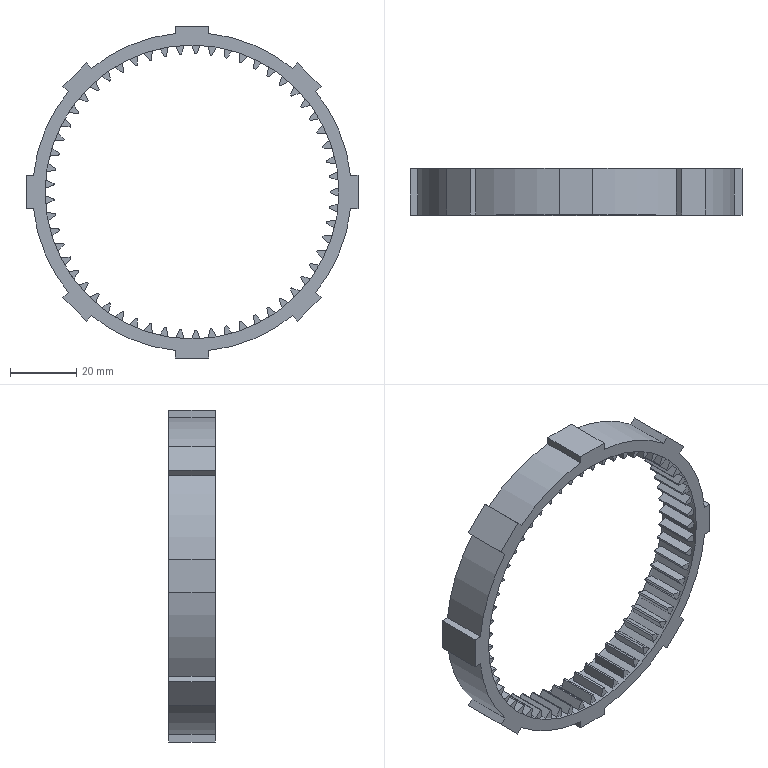Part | SolidWorks | features CirPattern 1, Extrusion 1, ICE 1 | 1 solid | 321 faces | box 100 x 14 x 100 mm | volume 20184 mm3 | plane 140 | spline 114 | cylinder 67 | commonest cylinder face diameters 83.25 x57 96 x8 88.5 x2